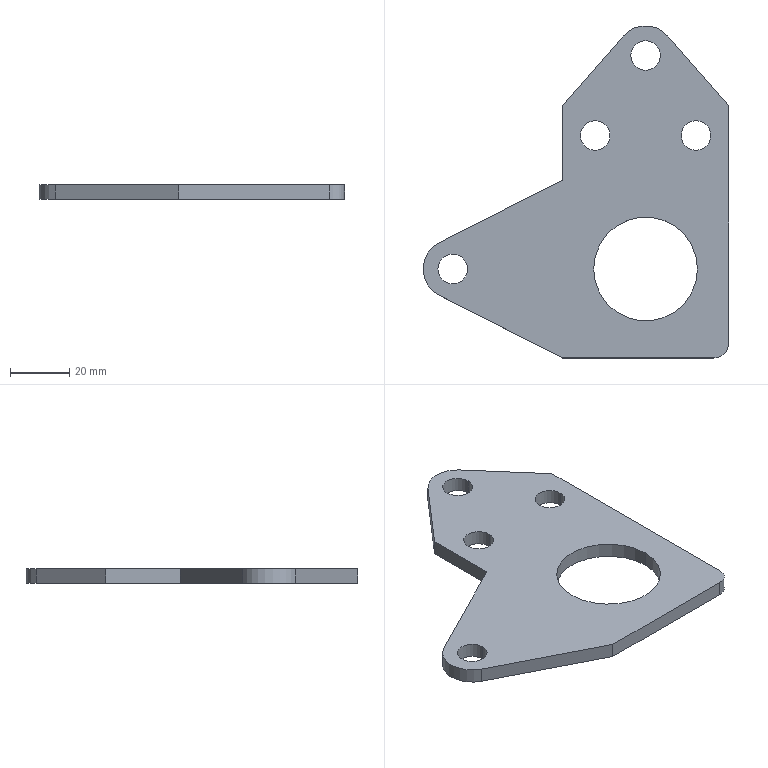Part | STEP file | MM-P46715-11_1 | 1 solid | 22 faces | box 103 x 112 x 5 mm | volume 30189 mm3 | cylinder 13 | plane 9 | commonest cylinder face diameters 10 x9 20 x2 35 x2